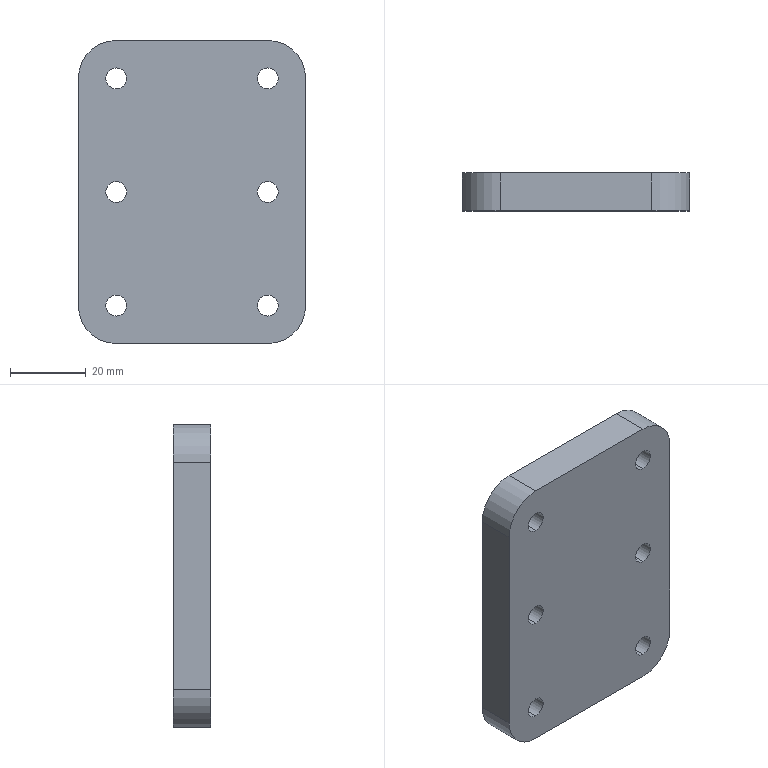Part | STEP file | PN_0021 | 1 solid | 40 faces | box 60 x 10 x 80 mm | volume 43843 mm3 | cylinder 28 | plane 12 | commonest cylinder face diameters 5.5 x12 10 x12 20 x4